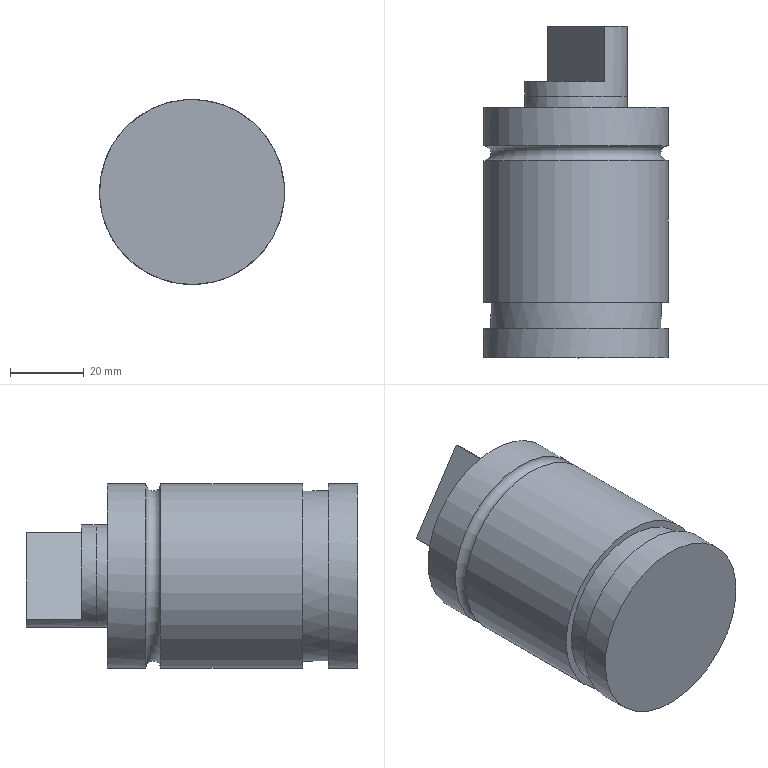Part | NX | features MAIN_BODY 2 | 1 solid | 16 faces | box 50.2 x 90 x 50.2 mm | volume 140216 mm3 | plane 8 | cylinder 7 | torus 1 | commonest cylinder face diameters 50.2 x3 6 x1 27.98 x1 28 x1 46.2 x1
STEP:
#1=CARTESIAN_POINT('',(-542.013,949.,-198.272));
#2=VERTEX_POINT('',#1);
#3=CARTESIAN_POINT('',(-521.,949.,-212.));
#4=DIRECTION('',(0.,1.,0.));
#5=DIRECTION('',(-0.8372,0.,0.5469));
#6=AXIS2_PLACEMENT_3D('',#3,#4,#5);
#7=CIRCLE('',#6,25.1);
#8=EDGE_CURVE('',#2,#2,#7,.F.);
#9=ORIENTED_EDGE('',*,*,#8,.F.);
#10=EDGE_LOOP('',(#9));
#11=FACE_BOUND('',#10,.T.);
#12=CARTESIAN_POINT('',(-542.013,987.5,-198.272));
#13=VERTEX_POINT('',#12);
#14=CARTESIAN_POINT('',(-521.,987.5,-212.));
#15=DIRECTION('',(0.,1.,0.));
#16=DIRECTION('',(-0.8372,0.,0.5469));
#17=AXIS2_PLACEMENT_3D('',#14,#15,#16);
#18=CIRCLE('',#17,25.1);
#19=EDGE_CURVE('',#13,#13,#18,.T.);
#20=ORIENTED_EDGE('',*,*,#19,.F.);
#21=EDGE_LOOP('',(#20));
#22=FACE_BOUND('',#21,.T.);
#23=CARTESIAN_POINT('',(-521.,1002.,-212.));
#24=DIRECTION('',(0.,-1.,0.));
#25=DIRECTION('',(-0.8372,0.,0.5469));
#26=AXIS2_PLACEMENT_3D('',#23,#24,#25);
#27=CYLINDRICAL_SURFACE('',#26,25.1);
#28=ADVANCED_FACE('',(#11,#22),#27,.T.);
#29=CARTESIAN_POINT('',(-499.987,1002.,-225.728));
#30=VERTEX_POINT('',#29);
#31=CARTESIAN_POINT('',(-521.,1002.,-212.));
#32=DIRECTION('',(0.,-1.,0.));
#33=DIRECTION('',(0.8372,0.,-0.5469));
#34=AXIS2_PLACEMENT_3D('',#31,#32,#33);
#35=CIRCLE('',#34,25.1);
#36=EDGE_CURVE('',#30,#30,#35,.T.);
#37=ORIENTED_EDGE('',*,*,#36,.F.);
#38=EDGE_LOOP('',(#37));
#39=FACE_BOUND('',#38,.T.);
#40=CARTESIAN_POINT('',(-509.28,1002.,-219.657));
#41=VERTEX_POINT('',#40);
#42=CARTESIAN_POINT('',(-521.,1002.,-212.));
#43=DIRECTION('',(0.,-1.,0.));
#44=DIRECTION('',(0.8372,0.,-0.5469));
#45=AXIS2_PLACEMENT_3D('',#42,#43,#44);
#46=CIRCLE('',#45,14.);
#47=EDGE_CURVE('',#41,#41,#46,.T.);
#48=ORIENTED_EDGE('',*,*,#47,.T.);
#49=EDGE_LOOP('',(#48));
#50=FACE_BOUND('',#49,.T.);
#51=CARTESIAN_POINT('',(-521.,1002.,-212.));
#52=DIRECTION('',(0.,1.,0.));
#53=DIRECTION('',(0.8372,0.,-0.5469));
#54=AXIS2_PLACEMENT_3D('',#51,#52,#53);
#55=PLANE('',#54);
#56=ADVANCED_FACE('',(#39,#50),#55,.T.);
#57=CARTESIAN_POINT('',(-542.013,991.5,-198.272));
#58=VERTEX_POINT('',#57);
#59=CARTESIAN_POINT('',(-521.,991.5,-212.));
#60=DIRECTION('',(0.,1.,0.));
#61=DIRECTION('',(-0.8372,0.,0.5469));
#62=AXIS2_PLACEMENT_3D('',#59,#60,#61);
#63=CIRCLE('',#62,25.1);
#64=EDGE_CURVE('',#58,#58,#63,.F.);
#65=ORIENTED_EDGE('',*,*,#64,.F.);
#66=EDGE_LOOP('',(#65));
#67=FACE_BOUND('',#66,.T.);
#68=ORIENTED_EDGE('',*,*,#36,.T.);
#69=EDGE_LOOP('',(#68));
#70=FACE_BOUND('',#69,.T.);
#71=CARTESIAN_POINT('',(-521.,1002.,-212.));
#72=DIRECTION('',(0.,-1.,0.));
#73=DIRECTION('',(-0.8372,0.,0.5469));
#74=AXIS2_PLACEMENT_3D('',#71,#72,#73);
#75=CYLINDRICAL_SURFACE('',#74,25.1);
#76=ADVANCED_FACE('',(#67,#70),#75,.T.);
#77=CARTESIAN_POINT('',(-518.146,1005.,-225.706));
#78=VERTEX_POINT('',#77);
#79=CARTESIAN_POINT('',(-508.023,1005.,-220.504));
#80=CARTESIAN_POINT('',(-517.837,1005.,-227.189));
#81=CARTESIAN_POINT('',(-529.504,1005.,-224.977));
#82=CARTESIAN_POINT('',(-536.189,1005.,-215.163));
#83=CARTESIAN_POINT('',(-533.977,1005.,-203.496));
#84=CARTESIAN_POINT('',(-524.163,1005.,-196.811));
#85=CARTESIAN_POINT('',(-512.496,1005.,-199.023));
#86=CARTESIAN_POINT('',(-505.811,1005.,-208.837));
#87=CARTESIAN_POINT('',(-508.023,1005.,-220.504));
#88=CARTESIAN_POINT('',(-517.837,1005.,-227.189));
#89=CARTESIAN_POINT('',(-529.504,1005.,-224.977));
#90=B_SPLINE_CURVE_WITH_KNOTS('',3,(#79,#80,#81,#82,#83,#84,#85,#86,#87,#88,#89),.UNSPECIFIED.,.T.,.F.,(1,1,1,1,1,1,1,1,1,1,1,1,1,1,1),(-0.2498,-0.1248,0.0002217,0.1252,0.2502,0.3752,0.5002,0.6252,0.7502,0.8752,1.,1.125,1.25,1.375,1.5),.UNSPECIFIED.);
#91=EDGE_CURVE('',#78,#78,#90,.F.);
#92=ORIENTED_EDGE('',*,*,#91,.T.);
#93=EDGE_LOOP('',(#92));
#94=FACE_BOUND('',#93,.T.);
#95=ORIENTED_EDGE('',*,*,#47,.F.);
#96=EDGE_LOOP('',(#95));
#97=FACE_BOUND('',#96,.T.);
#98=CARTESIAN_POINT('',(-521.,1005.,-212.));
#99=DIRECTION('',(0.,-1.,0.));
#100=DIRECTION('',(-0.8372,0.,0.5469));
#101=AXIS2_PLACEMENT_3D('',#98,#99,#100);
#102=CYLINDRICAL_SURFACE('',#101,14.);
#103=ADVANCED_FACE('',(#94,#97),#102,.T.);
#104=ORIENTED_EDGE('',*,*,#64,.T.);
#105=EDGE_LOOP('',(#104));
#106=FACE_BOUND('',#105,.T.);
#107=ORIENTED_EDGE('',*,*,#19,.T.);
#108=EDGE_LOOP('',(#107));
#109=FACE_BOUND('',#108,.T.);
#110=CARTESIAN_POINT('',(-521.,989.5,-212.));
#111=DIRECTION('',(0.,-1.,0.));
#112=DIRECTION('',(-0.8372,0.,0.5469));
#113=AXIS2_PLACEMENT_3D('',#110,#111,#112);
#114=TOROIDAL_SURFACE('',#113,25.1,2.);
#115=ADVANCED_FACE('',(#106,#109),#114,.F.);
#116=CARTESIAN_POINT('',(-501.661,949.,-224.634));
#117=VERTEX_POINT('',#116);
#118=CARTESIAN_POINT('',(-521.,949.,-212.));
#119=DIRECTION('',(0.,-1.,0.));
#120=DIRECTION('',(0.8372,0.,-0.5469));
#121=AXIS2_PLACEMENT_3D('',#118,#119,#120);
#122=CIRCLE('',#121,23.1);
#123=EDGE_CURVE('',#117,#117,#122,.T.);
#124=ORIENTED_EDGE('',*,*,#123,.F.);
#125=EDGE_LOOP('',(#124));
#126=FACE_BOUND('',#125,.T.);
#127=ORIENTED_EDGE('',*,*,#8,.T.);
#128=EDGE_LOOP('',(#127));
#129=FACE_BOUND('',#128,.T.);
#130=CARTESIAN_POINT('',(-521.,949.,-212.));
#131=DIRECTION('',(0.,-1.,0.));
#132=DIRECTION('',(-0.8372,0.,0.5469));
#133=AXIS2_PLACEMENT_3D('',#130,#131,#132);
#134=PLANE('',#133);
#135=ADVANCED_FACE('',(#126,#129),#134,.T.);
#136=CARTESIAN_POINT('',(-500.529,942.,-222.703));
#137=VERTEX_POINT('',#136);
#138=CARTESIAN_POINT('',(-502.975,942.,-226.447));
#139=VERTEX_POINT('',#138);
#140=CARTESIAN_POINT('',(-521.,942.,-212.));
#141=DIRECTION('',(0.,-1.,0.));
#142=DIRECTION('',(0.8372,0.,-0.5469));
#143=AXIS2_PLACEMENT_3D('',#140,#141,#142);
#144=CIRCLE('',#143,23.1);
#145=EDGE_CURVE('',#137,#139,#144,.T.);
#146=ORIENTED_EDGE('',*,*,#145,.T.);
#147=CARTESIAN_POINT('',(-501.294,942.,-227.546));
#148=VERTEX_POINT('',#147);
#149=CARTESIAN_POINT('',(-507.489,942.,-223.498));
#150=DIRECTION('',(0.8372,0.,-0.5469));
#151=VECTOR('',#150,1000.);
#152=LINE('',#149,#151);
#153=EDGE_CURVE('',#148,#139,#152,.F.);
#154=ORIENTED_EDGE('',*,*,#153,.F.);
#155=CARTESIAN_POINT('',(-498.848,942.,-223.802));
#156=VERTEX_POINT('',#155);
#157=CARTESIAN_POINT('',(-521.,942.,-212.));
#158=DIRECTION('',(0.,1.,0.));
#159=DIRECTION('',(-0.8372,0.,0.5469));
#160=AXIS2_PLACEMENT_3D('',#157,#158,#159);
#161=CIRCLE('',#160,25.1);
#162=EDGE_CURVE('',#148,#156,#161,.T.);
#163=ORIENTED_EDGE('',*,*,#162,.T.);
#164=CARTESIAN_POINT('',(-505.043,942.,-219.754));
#165=DIRECTION('',(0.8372,0.,-0.5469));
#166=VECTOR('',#165,1000.);
#167=LINE('',#164,#166);
#168=EDGE_CURVE('',#137,#156,#167,.T.);
#169=ORIENTED_EDGE('',*,*,#168,.F.);
#170=EDGE_LOOP('',(#146,#154,#163,#169));
#171=FACE_BOUND('',#170,.T.);
#172=CARTESIAN_POINT('',(-521.,942.,-212.));
#173=DIRECTION('',(0.,-1.,0.));
#174=DIRECTION('',(-0.8372,0.,0.5469));
#175=AXIS2_PLACEMENT_3D('',#172,#173,#174);
#176=PLANE('',#175);
#177=ADVANCED_FACE('',(#171),#176,.F.);
#178=CARTESIAN_POINT('',(-500.529,942.,-222.703));
#179=CARTESIAN_POINT('',(-500.792,942.632,-223.207));
#180=CARTESIAN_POINT('',(-501.617,943.368,-224.664));
#181=CARTESIAN_POINT('',(-502.62,942.632,-226.004));
#182=CARTESIAN_POINT('',(-502.975,942.,-226.447));
#183=B_SPLINE_CURVE_WITH_KNOTS('',3,(#178,#179,#180,#181,#182),.UNSPECIFIED.,.F.,.F.,(4,1,4),(0.,0.002514,0.005028),.UNSPECIFIED.);
#184=EDGE_CURVE('',#137,#139,#183,.T.);
#185=ORIENTED_EDGE('',*,*,#184,.T.);
#186=ORIENTED_EDGE('',*,*,#145,.F.);
#187=EDGE_LOOP('',(#185,#186));
#188=FACE_BOUND('',#187,.T.);
#189=ORIENTED_EDGE('',*,*,#123,.T.);
#190=EDGE_LOOP('',(#189));
#191=FACE_BOUND('',#190,.T.);
#192=CARTESIAN_POINT('',(-521.,942.,-212.));
#193=DIRECTION('',(0.,1.,0.));
#194=DIRECTION('',(0.8372,0.,-0.5469));
#195=AXIS2_PLACEMENT_3D('',#192,#193,#194);
#196=CYLINDRICAL_SURFACE('',#195,23.1);
#197=ADVANCED_FACE('',(#188,#191),#196,.T.);
#198=CARTESIAN_POINT('',(-499.987,934.,-225.728));
#199=VERTEX_POINT('',#198);
#200=CARTESIAN_POINT('',(-521.,934.,-212.));
#201=DIRECTION('',(0.,-1.,0.));
#202=DIRECTION('',(0.8372,0.,-0.5469));
#203=AXIS2_PLACEMENT_3D('',#200,#201,#202);
#204=CIRCLE('',#203,25.1);
#205=EDGE_CURVE('',#199,#199,#204,.T.);
#206=ORIENTED_EDGE('',*,*,#205,.T.);
#207=EDGE_LOOP('',(#206));
#208=FACE_BOUND('',#207,.T.);
#209=CARTESIAN_POINT('',(-521.,934.,-212.));
#210=DIRECTION('',(0.,1.,0.));
#211=DIRECTION('',(0.8372,0.,-0.5469));
#212=AXIS2_PLACEMENT_3D('',#209,#210,#211);
#213=PLANE('',#212);
#214=ADVANCED_FACE('',(#208),#213,.F.);
#215=ORIENTED_EDGE('',*,*,#162,.F.);
#216=CARTESIAN_POINT('',(-498.848,942.,-223.802));
#217=CARTESIAN_POINT('',(-498.483,941.135,-223.117));
#218=CARTESIAN_POINT('',(-498.306,938.482,-222.761));
#219=CARTESIAN_POINT('',(-499.895,936.26,-225.783));
#220=CARTESIAN_POINT('',(-502.029,938.479,-228.461));
#221=CARTESIAN_POINT('',(-501.774,941.135,-228.155));
#222=CARTESIAN_POINT('',(-501.294,942.,-227.546));
#223=B_SPLINE_CURVE_WITH_KNOTS('',3,(#216,#217,#218,#219,#220,#221,#222),.UNSPECIFIED.,.F.,.F.,(4,1,1,1,4),(0.,0.003437,0.006873,0.01031,0.01375),.UNSPECIFIED.);
#224=EDGE_CURVE('',#156,#148,#223,.T.);
#225=ORIENTED_EDGE('',*,*,#224,.F.);
#226=EDGE_LOOP('',(#215,#225));
#227=FACE_BOUND('',#226,.T.);
#228=ORIENTED_EDGE('',*,*,#205,.F.);
#229=EDGE_LOOP('',(#228));
#230=FACE_BOUND('',#229,.T.);
#231=CARTESIAN_POINT('',(-521.,988.,-212.));
#232=DIRECTION('',(0.,-1.,0.));
#233=DIRECTION('',(-0.8372,0.,0.5469));
#234=AXIS2_PLACEMENT_3D('',#231,#232,#233);
#235=CYLINDRICAL_SURFACE('',#234,25.1);
#236=ADVANCED_FACE('',(#227,#230),#235,.T.);
#237=ORIENTED_EDGE('',*,*,#184,.F.);
#238=ORIENTED_EDGE('',*,*,#168,.T.);
#239=ORIENTED_EDGE('',*,*,#224,.T.);
#240=ORIENTED_EDGE('',*,*,#153,.T.);
#241=EDGE_LOOP('',(#237,#238,#239,#240));
#242=FACE_BOUND('',#241,.T.);
#243=CARTESIAN_POINT('',(-504.625,940.,-219.115));
#244=VERTEX_POINT('',#243);
#245=CARTESIAN_POINT('',(-506.266,940.,-221.626));
#246=DIRECTION('',(-0.8372,0.,0.5469));
#247=DIRECTION('',(0.5469,0.,0.8372));
#248=AXIS2_PLACEMENT_3D('',#245,#246,#247);
#249=CIRCLE('',#248,3.);
#250=EDGE_CURVE('',#244,#244,#249,.T.);
#251=ORIENTED_EDGE('',*,*,#250,.T.);
#252=EDGE_LOOP('',(#251));
#253=FACE_BOUND('',#252,.T.);
#254=CARTESIAN_POINT('',(-506.266,940.,-221.626));
#255=DIRECTION('',(0.8372,0.,-0.5469));
#256=DIRECTION('',(0.,-1.,0.));
#257=AXIS2_PLACEMENT_3D('',#254,#255,#256);
#258=CYLINDRICAL_SURFACE('',#257,3.);
#259=ADVANCED_FACE('',(#242,#253),#258,.F.);
#260=ORIENTED_EDGE('',*,*,#250,.F.);
#261=EDGE_LOOP('',(#260));
#262=FACE_BOUND('',#261,.T.);
#263=CARTESIAN_POINT('',(-506.266,940.,-221.626));
#264=DIRECTION('',(0.8372,0.,-0.5469));
#265=DIRECTION('',(0.,-1.,0.));
#266=AXIS2_PLACEMENT_3D('',#263,#264,#265);
#267=PLANE('',#266);
#268=ADVANCED_FACE('',(#262),#267,.T.);
#269=ORIENTED_EDGE('',*,*,#91,.F.);
#270=EDGE_LOOP('',(#269));
#271=FACE_BOUND('',#270,.T.);
#272=CARTESIAN_POINT('',(-513.343,1024.,-200.28));
#273=VERTEX_POINT('',#272);
#274=CARTESIAN_POINT('',(-513.343,1009.,-200.28));
#275=VERTEX_POINT('',#274);
#276=CARTESIAN_POINT('',(-513.348,1024.,-200.288));
#277=DIRECTION('',(0.,-1.,0.));
#278=VECTOR('',#277,1000.);
#279=LINE('',#276,#278);
#280=EDGE_CURVE('',#273,#275,#279,.T.);
#281=ORIENTED_EDGE('',*,*,#280,.T.);
#282=CARTESIAN_POINT('',(-528.657,1009.,-223.72));
#283=VERTEX_POINT('',#282);
#284=CARTESIAN_POINT('',(-521.,1009.,-212.));
#285=DIRECTION('',(0.,1.,0.));
#286=DIRECTION('',(-0.8372,0.,0.5469));
#287=AXIS2_PLACEMENT_3D('',#284,#285,#286);
#288=CIRCLE('',#287,13.99);
#289=EDGE_CURVE('',#283,#275,#288,.T.);
#290=ORIENTED_EDGE('',*,*,#289,.F.);
#291=CARTESIAN_POINT('',(-528.657,1024.,-223.72));
#292=VERTEX_POINT('',#291);
#293=CARTESIAN_POINT('',(-528.652,1009.,-223.712));
#294=DIRECTION('',(0.,-1.,0.));
#295=VECTOR('',#294,1000.);
#296=LINE('',#293,#295);
#297=EDGE_CURVE('',#283,#292,#296,.F.);
#298=ORIENTED_EDGE('',*,*,#297,.T.);
#299=CARTESIAN_POINT('',(-521.,1024.,-212.));
#300=DIRECTION('',(0.,-1.,0.));
#301=DIRECTION('',(0.8372,0.,-0.5469));
#302=AXIS2_PLACEMENT_3D('',#299,#300,#301);
#303=CIRCLE('',#302,13.99);
#304=EDGE_CURVE('',#292,#273,#303,.T.);
#305=ORIENTED_EDGE('',*,*,#304,.T.);
#306=EDGE_LOOP('',(#281,#290,#298,#305));
#307=FACE_BOUND('',#306,.T.);
#308=CARTESIAN_POINT('',(-521.,1024.,-212.));
#309=DIRECTION('',(0.,-1.,0.));
#310=DIRECTION('',(-0.8372,0.,0.5469));
#311=AXIS2_PLACEMENT_3D('',#308,#309,#310);
#312=CYLINDRICAL_SURFACE('',#311,13.99);
#313=ADVANCED_FACE('',(#271,#307),#312,.T.);
#314=ORIENTED_EDGE('',*,*,#304,.F.);
#315=CARTESIAN_POINT('',(-421.345,1024.,-59.466));
#316=DIRECTION('',(-0.5469,0.,-0.8372));
#317=VECTOR('',#316,1000.);
#318=LINE('',#315,#317);
#319=EDGE_CURVE('',#273,#292,#318,.T.);
#320=ORIENTED_EDGE('',*,*,#319,.F.);
#321=EDGE_LOOP('',(#314,#320));
#322=FACE_BOUND('',#321,.T.);
#323=CARTESIAN_POINT('',(-521.,1024.,-212.));
#324=DIRECTION('',(0.,1.,0.));
#325=DIRECTION('',(0.8372,0.,-0.5469));
#326=AXIS2_PLACEMENT_3D('',#323,#324,#325);
#327=PLANE('',#326);
#328=ADVANCED_FACE('',(#322),#327,.T.);
#329=CARTESIAN_POINT('',(-421.345,1009.,-59.466));
#330=DIRECTION('',(-0.5469,0.,-0.8372));
#331=VECTOR('',#330,1000.);
#332=LINE('',#329,#331);
#333=EDGE_CURVE('',#275,#283,#332,.T.);
#334=ORIENTED_EDGE('',*,*,#333,.T.);
#335=ORIENTED_EDGE('',*,*,#289,.T.);
#336=EDGE_LOOP('',(#334,#335));
#337=FACE_BOUND('',#336,.T.);
#338=CARTESIAN_POINT('',(-421.345,1009.,-59.466));
#339=DIRECTION('',(0.,-1.,0.));
#340=DIRECTION('',(-0.8372,0.,0.5469));
#341=AXIS2_PLACEMENT_3D('',#338,#339,#340);
#342=PLANE('',#341);
#343=ADVANCED_FACE('',(#337),#342,.F.);
#344=ORIENTED_EDGE('',*,*,#280,.F.);
#345=ORIENTED_EDGE('',*,*,#319,.T.);
#346=ORIENTED_EDGE('',*,*,#297,.F.);
#347=ORIENTED_EDGE('',*,*,#333,.F.);
#348=EDGE_LOOP('',(#344,#345,#346,#347));
#349=FACE_BOUND('',#348,.T.);
#350=CARTESIAN_POINT('',(-421.345,1009.,-59.466));
#351=DIRECTION('',(-0.8372,0.,0.5469));
#352=DIRECTION('',(-0.5469,0.,-0.8372));
#353=AXIS2_PLACEMENT_3D('',#350,#351,#352);
#354=PLANE('',#353);
#355=ADVANCED_FACE('',(#349),#354,.T.);
#356=CLOSED_SHELL('',(#28,#56,#76,#103,#115,#135,#177,#197,#214,#236,#259,#268,#313,#328,#343,#355));
#357=MANIFOLD_SOLID_BREP('',#356);
#358=(LENGTH_UNIT()NAMED_UNIT(*)SI_UNIT(.MILLI.,.METRE.));
#359=UNCERTAINTY_MEASURE_WITH_UNIT(LENGTH_MEASURE(0.0508),#358,'','');
#360=(NAMED_UNIT(*)PLANE_ANGLE_UNIT()SI_UNIT($,.RADIAN.));
#361=(NAMED_UNIT(*)SI_UNIT($,.STERADIAN.)SOLID_ANGLE_UNIT());
#362=(GEOMETRIC_REPRESENTATION_CONTEXT(3)GLOBAL_UNCERTAINTY_ASSIGNED_CONTEXT((#359))GLOBAL_UNIT_ASSIGNED_CONTEXT((#358,#360,#361))REPRESENTATION_CONTEXT('',''));
#363=ADVANCED_BREP_SHAPE_REPRESENTATION('',(#357),#362);